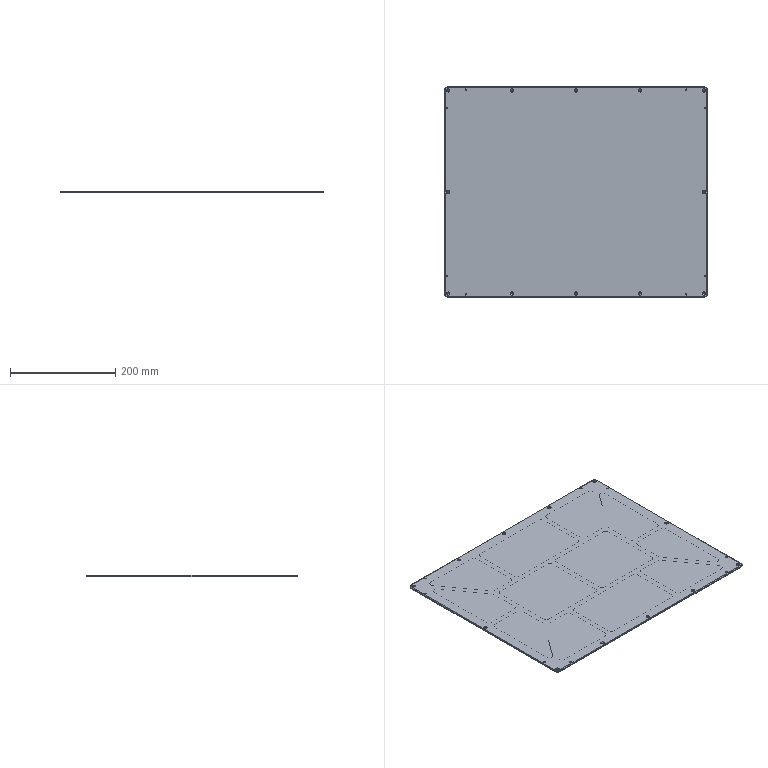NC program | Mastercam | posted with a generic post | part box 500 x 400 x 3 mm
Lines 11032 to 11256 of 11256:
(4 CHM |TOOL - 5|DIA. OFF. - 5|LEN. - 5|TOOL DIA. - 4.)
N2336 T5 M6
N2338 G0 G54 G90 X-101.1 Y178.55 C0. B0. S7000 M3
N2340 G43 H5 Z50.
N2342 Z1.
N2344 G1 Z-.7 F600.
N2346 Y178.95 F1000.
N2348 G3 X-101.5 Y179.35 I-.4
N2350 G1 X-211.053
N2352 G3 X-216.903 Y173.5 J-5.85
N2354 X-215.784 Y170.059 I5.85
N2356 G1 X-148.875 Y78.059
N2358 G3 X-144.144 Y75.65 I4.731 J3.441
N2360 G1 X-101.5
N2362 G3 X-95.65 Y81.5 J5.85
N2364 G1 Y173.5
N2366 G3 X-101.5 Y179.35 I-5.85
N2368 G1 X-102.
N2370 G3 X-102.4 Y178.95 J-.4
N2372 G1 Y178.55
N2374 G0 Z50.
N2376 X78.9
N2378 Z1.
N2380 G1 Z-.7 F600.
N2382 Y178.95 F1000.
N2384 G3 X78.5 Y179.35 I-.4
N2386 G1 X-78.5
N2388 G3 X-84.35 Y173.5 J-5.85
N2390 G1 Y81.5
N2392 G3 X-78.5 Y75.65 I5.85
N2394 G1 X78.5
N2396 G3 X84.35 Y81.5 J5.85
N2398 G1 Y173.5
N2400 G3 X78.5 Y179.35 I-5.85
N2402 G1 X78.
N2404 G3 X77.6 Y178.95 J-.4
N2406 G1 Y178.55
N2408 G0 Z50.
N2410 X211.453
N2412 Z1.
N2414 G1 Z-.7 F600.
N2416 Y178.95 F1000.
N2418 G3 X211.053 Y179.35 I-.4
N2420 G1 X101.5
N2422 G3 X95.65 Y173.5 J-5.85
N2424 G1 Y81.5
N2426 G3 X101.5 Y75.65 I5.85
N2428 G1 X144.144
N2430 G3 X148.875 Y78.059 J5.85
N2432 G1 X215.784 Y170.059
N2434 G3 X216.903 Y173.5 I-4.731 J3.441
N2436 X211.053 Y179.35 I-5.85
N2438 G1 X210.553
N2440 G3 X210.153 Y178.95 J-.4
N2442 G1 Y178.55
N2444 G0 Z50.
N2446 X219.651 Y154.804
N2448 Z1.
N2450 G1 Z-.7 F600.
N2452 X219.328 Y155.039 F1000.
N2454 G3 X219.092 Y155.116 I-.236 J-.323
N2456 X218.769 Y154.951 J-.4
N2458 G1 X156.769 Y69.701
N2460 G3 X155.65 Y66.26 I4.731 J-3.441
N2462 G1 Y11.5
N2464 G3 X161.5 Y5.65 I5.85
N2466 G1 X223.5
N2468 G3 X229.35 Y11.5 J5.85
N2470 G1 Y151.51
N2472 G3 X223.5 Y157.36 I-5.85
N2474 X218.769 Y154.951 J-5.85
N2476 G1 X218.475 Y154.547
N2478 G3 X218.399 Y154.312 I.323 J-.235
N2480 X218.563 Y153.988 I.399
N2482 G1 X218.887 Y153.753
N2484 G0 Z50.
N2486 X138.9 Y63.55
N2488 Z1.
N2490 G1 Z-.7 F600.
N2492 Y63.95 F1000.
N2494 G3 X138.5 Y64.35 I-.4
N2496 G1 X11.5
N2498 G3 X5.65 Y58.5 J-5.85
N2500 G1 Y-58.5
N2502 G3 X11.5 Y-64.35 I5.85
N2504 G1 X138.5
N2506 G3 X144.35 Y-58.5 J5.85
N2508 G1 Y58.5
N2510 G3 X138.5 Y64.35 I-5.85
N2512 G1 X138.
N2514 G3 X137.6 Y63.95 J-.4
N2516 G1 Y63.55
N2518 G0 Z50.
N2520 X-11.1
N2522 Z1.
N2524 G1 Z-.7 F600.
N2526 Y63.95 F1000.
N2528 G3 X-11.5 Y64.35 I-.4
N2530 G1 X-138.5
N2532 G3 X-144.35 Y58.5 J-5.85
N2534 G1 Y-58.5
N2536 G3 X-138.5 Y-64.35 I5.85
N2538 G1 X-11.5
N2540 G3 X-5.65 Y-58.5 J5.85
N2542 G1 Y58.5
N2544 G3 X-11.5 Y64.35 I-5.85
N2546 G1 X-12.
N2548 G3 X-12.4 Y63.95 J-.4
N2550 G1 Y63.55
N2552 G0 Z50.
N2554 X-157.181 Y68.907
N2556 Z1.
N2558 G1 Z-.7 F600.
N2560 X-156.857 Y69.142 F1000.
N2562 G3 X-156.692 Y69.466 I-.235 J.324
N2564 X-156.769 Y69.701 I-.4
N2566 G1 X-218.769 Y154.951
N2568 G3 X-223.5 Y157.36 I-4.731 J-3.441
N2570 X-229.35 Y151.51 J-5.85
N2572 G1 Y11.5
N2574 G3 X-223.5 Y5.65 I5.85
N2576 G1 X-161.5
N2578 G3 X-155.65 Y11.5 J5.85
N2580 G1 Y66.26
N2582 G3 X-156.769 Y69.701 I-5.85
N2584 G1 X-157.063 Y70.106
N2586 G3 X-157.386 Y70.27 I-.323 J-.236
N2588 X-157.622 Y70.194 J-.4
N2590 G1 X-157.945 Y69.959
N2592 G0 Z50.
N2594 X-161.1 Y-6.45
N2596 Z1.
N2598 G1 Z-.7 F600.
N2600 Y-6.05 F1000.
N2602 G3 X-161.5 Y-5.65 I-.4
N2604 G1 X-223.5
N2606 G3 X-229.35 Y-11.5 J-5.85
N2608 G1 Y-151.51
N2610 G3 X-223.5 Y-157.36 I5.85
N2612 X-218.769 Y-154.951 J5.85
N2614 G1 X-156.769 Y-69.701
N2616 G3 X-155.65 Y-66.26 I-4.731 J3.441
N2618 G1 Y-11.5
N2620 G3 X-161.5 Y-5.65 I-5.85
N2622 G1 X-162.
N2624 G3 X-162.4 Y-6.05 J-.4
N2626 G1 Y-6.45
N2628 G0 Z50.
N2630 X-101.1 Y-76.45
N2632 Z1.
N2634 G1 Z-.7 F600.
N2636 Y-76.05 F1000.
N2638 G3 X-101.5 Y-75.65 I-.4
N2640 G1 X-144.144
N2642 G3 X-148.875 Y-78.059 J-5.85
N2644 G1 X-215.784 Y-170.059
N2646 G3 X-216.903 Y-173.5 I4.731 J-3.441
N2648 X-211.053 Y-179.35 I5.85
N2650 G1 X-101.5
N2652 G3 X-95.65 Y-173.5 J5.85
N2654 G1 Y-81.5
N2656 G3 X-101.5 Y-75.65 I-5.85
N2658 G1 X-102.
N2660 G3 X-102.4 Y-76.05 J-.4
N2662 G1 Y-76.45
N2664 G0 Z50.
N2666 X78.9
N2668 Z1.
N2670 G1 Z-.7 F600.
N2672 Y-76.05 F1000.
N2674 G3 X78.5 Y-75.65 I-.4
N2676 G1 X-78.5
N2678 G3 X-84.35 Y-81.5 J-5.85
N2680 G1 Y-173.5
N2682 G3 X-78.5 Y-179.35 I5.85
N2684 G1 X78.5
N2686 G3 X84.35 Y-173.5 J5.85
N2688 G1 Y-81.5
N2690 G3 X78.5 Y-75.65 I-5.85
N2692 G1 X78.
N2694 G3 X77.6 Y-76.05 J-.4
N2696 G1 Y-76.45
N2698 G0 Z50.
N2700 X144.544
N2702 Z1.
N2704 G1 Z-.7 F600.
N2706 Y-76.05 F1000.
N2708 G3 X144.144 Y-75.65 I-.4
N2710 G1 X101.5
N2712 G3 X95.65 Y-81.5 J-5.85
N2714 G1 Y-173.5
N2716 G3 X101.5 Y-179.35 I5.85
N2718 G1 X211.053
N2720 G3 X216.903 Y-173.5 J5.85
N2722 X215.784 Y-170.059 I-5.85
N2724 G1 X148.875 Y-78.059
N2726 G3 X144.144 Y-75.65 I-4.731 J-3.441
N2728 G1 X143.644
N2730 G3 X143.244 Y-76.05 J-.4
N2732 G1 Y-76.45
N2734 G0 Z50.
N2736 X223.9 Y-6.45
N2738 Z1.
N2740 G1 Z-.7 F600.
N2742 Y-6.05 F1000.
N2744 G3 X223.5 Y-5.65 I-.4
N2746 G1 X161.5
N2748 G3 X155.65 Y-11.5 J-5.85
N2750 G1 Y-66.26
N2752 G3 X156.769 Y-69.701 I5.85
N2754 G1 X218.769 Y-154.951
N2756 G3 X223.5 Y-157.36 I4.731 J3.441
N2758 X229.35 Y-151.51 J5.85
N2760 G1 Y-11.5
N2762 G3 X223.5 Y-5.65 I-5.85
N2764 G1 X223.
N2766 G3 X222.6 Y-6.05 J-.4
N2768 G1 Y-6.45
N2770 G0 Z50.
N2772 M5
N2774 G0 G28 G91 Z0.
N2776 G0 G28 X0. Y0.
N2778 G28
N2780 M30
%